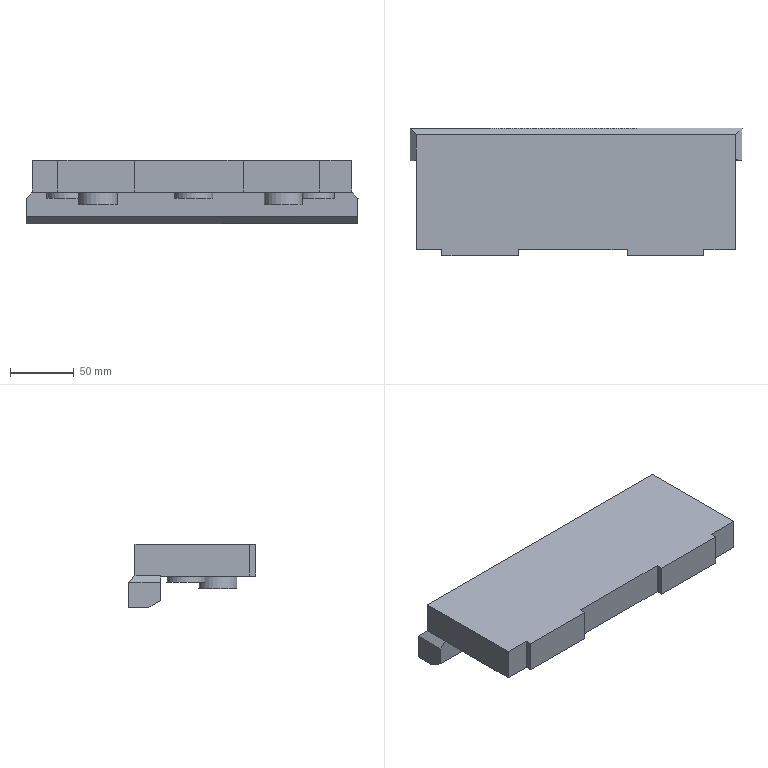Part | NX | features solid 2 | 1 solid | 33 faces | box 260 x 100.165 x 49.894 mm | volume 752244 mm3 | plane 22 | spline 6 | cylinder 5 | commonest cylinder face diameters 30 x5